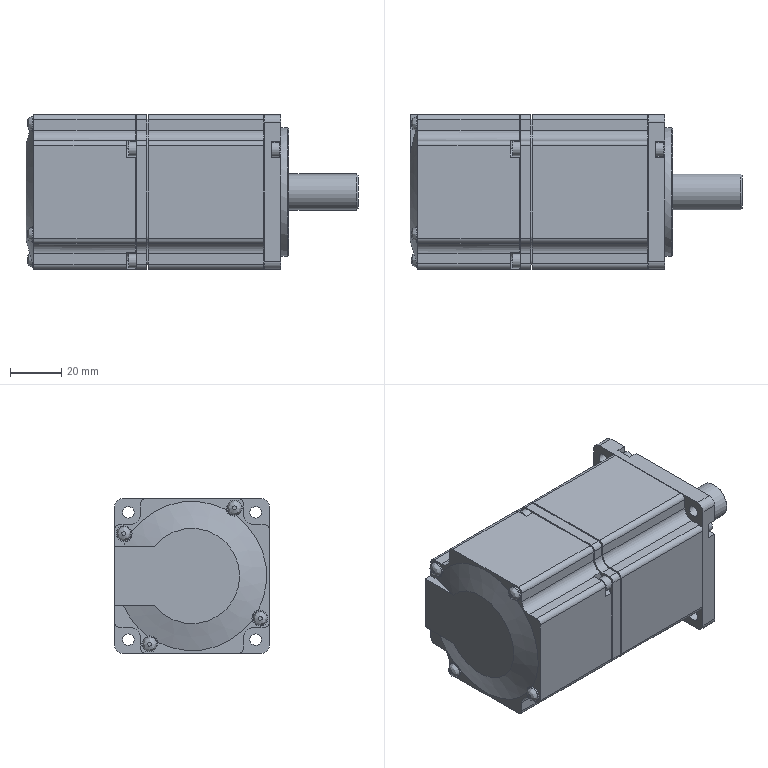Part | NX | 1 solid | 243 faces | box 129 x 60 x 60 mm | volume 323840 mm3 | plane 133 | cylinder 103 | spline 4 | cone 3 | commonest cylinder face diameters 4 x44 8 x24 6.5 x12 5.5 x8 6 x8 4.5 x4